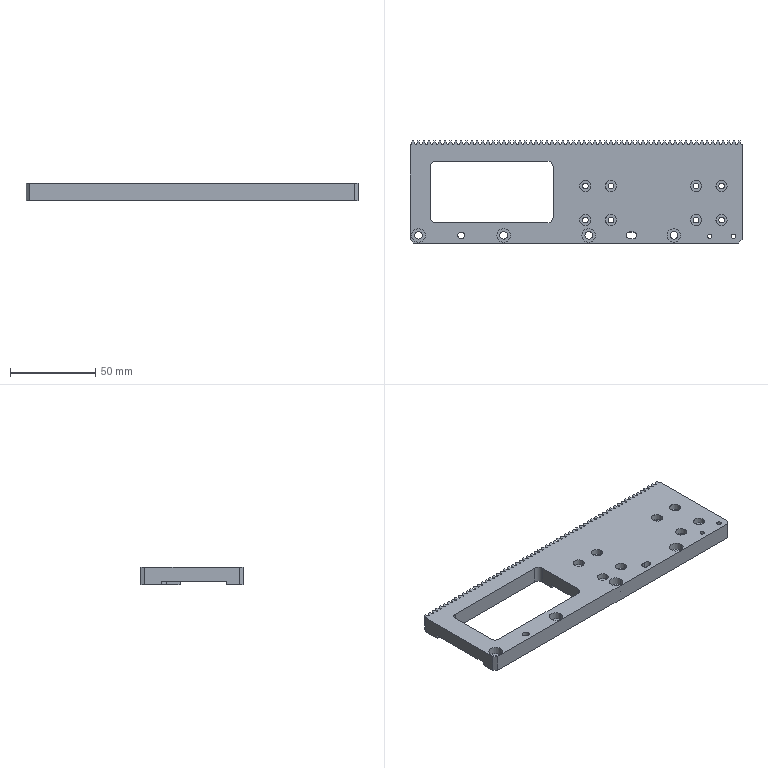Part | STEP file | QA-AD08 | 1 solid | 480 faces | box 195 x 60 x 10 mm | volume 78945 mm3 | plane 278 | cylinder 186 | cone 16 | commonest cylinder face diameters 0.6 x125 3.4 x16 6.5 x16 4.5 x8 8 x8 4 x5